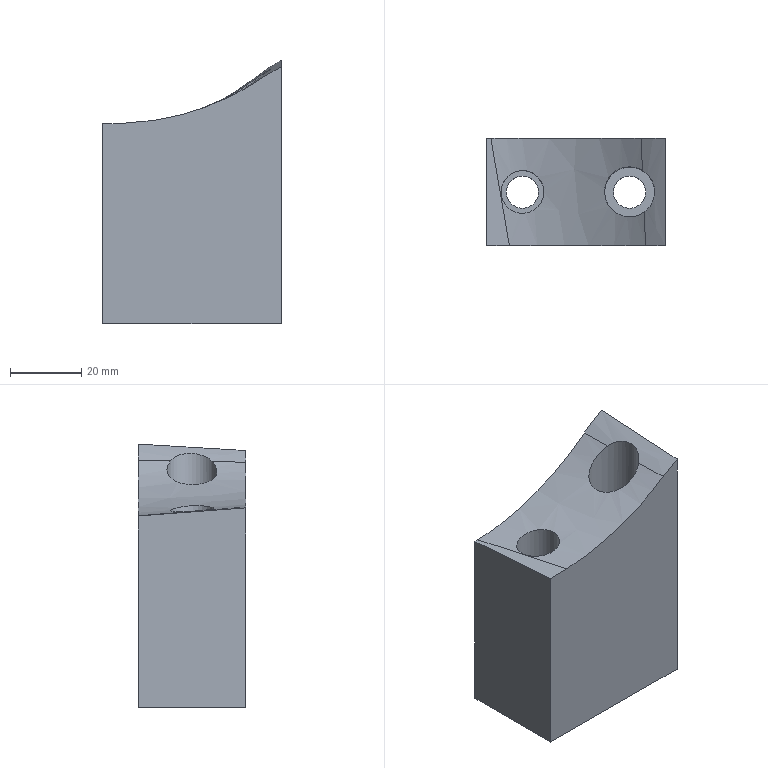Part | NX | features solid 2 | 1 solid | 14 faces | box 50 x 30.002 x 73.834 mm | volume 76103 mm3 | plane 7 | cylinder 4 | spline 3 | commonest cylinder face diameters 9 x2 12 x1 14 x1